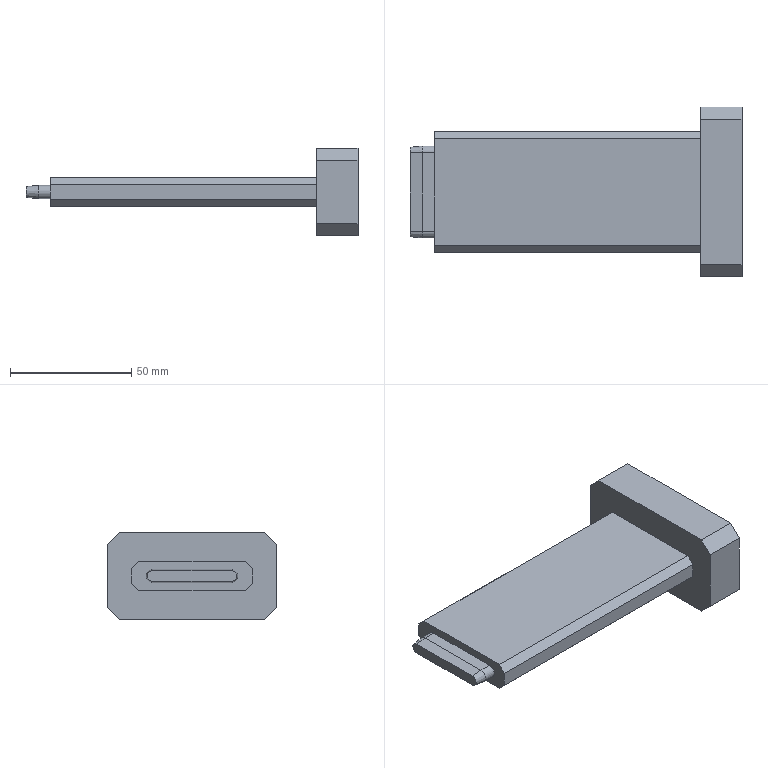Part | STEP file | Tube feed_id618_x_t | 1 solid | 28 faces | box 137 x 70 x 36 mm | volume 107934 mm3 | plane 24 | cylinder 2 | cone 2 | commonest cylinder face diameters 5.5 x2